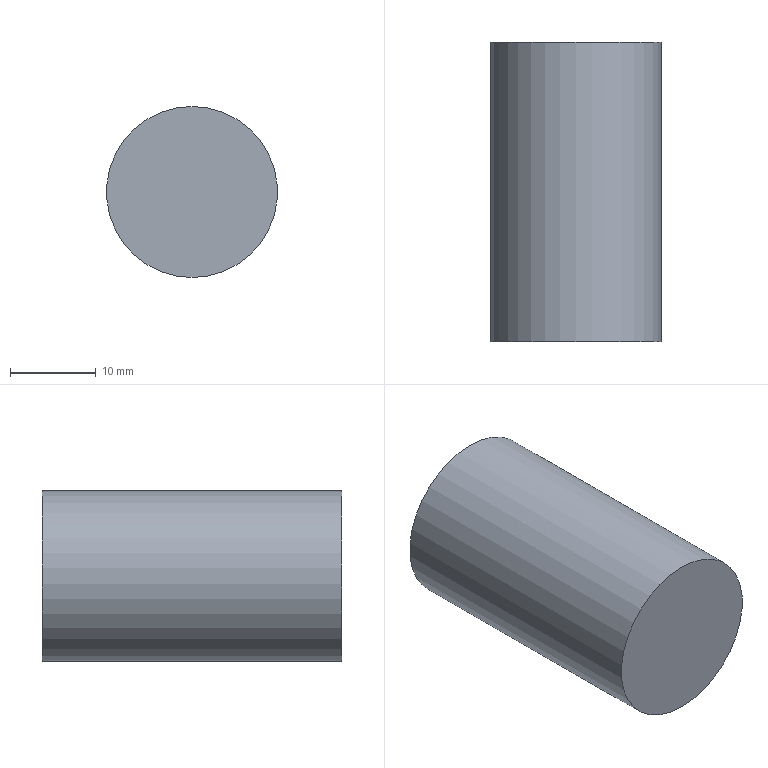Part | STEP file | dijiaolianjie | 1 solid | 3 faces | box 20 x 35 x 20 mm | volume 10996 mm3 | plane 2 | cylinder 1 | commonest cylinder face diameters 20 x1
STEP:
#1=CARTESIAN_POINT('',(0.,0.,0.));
#2=DIRECTION('',(0.,0.,1.));
#3=DIRECTION('',(1.,0.,0.));
#4=AXIS2_PLACEMENT_3D('',#1,#2,#3);
#5=CARTESIAN_POINT('',(0.,35.,10.));
#6=VERTEX_POINT('',#5);
#7=CARTESIAN_POINT('',(0.,35.,0.));
#8=DIRECTION('',(0.,1.,0.));
#9=DIRECTION('',(0.,0.,1.));
#10=AXIS2_PLACEMENT_3D('',#7,#8,#9);
#11=CIRCLE('',#10,10.);
#12=CARTESIAN_POINT('',(0.,35.,0.));
#13=DIRECTION('',(0.,-1.,0.));
#14=DIRECTION('',(0.,0.,-1.));
#15=AXIS2_PLACEMENT_3D('',#12,#13,#14);
#16=CYLINDRICAL_SURFACE('',#15,10.);
#17=CARTESIAN_POINT('',(9.425,0.));
#18=DIRECTION('',(-1.,0.));
#19=VECTOR('',#18,1.);
#20=LINE('',#17,#19);
#21=(GEOMETRIC_REPRESENTATION_CONTEXT(2)PARAMETRIC_REPRESENTATION_CONTEXT()REPRESENTATION_CONTEXT('',''));
#22=DEFINITIONAL_REPRESENTATION('',(#20),#21);
#23=PCURVE('',#16,#22);
#24=CARTESIAN_POINT('',(0.,35.,0.));
#25=DIRECTION('',(0.,1.,0.));
#26=DIRECTION('',(0.,0.,1.));
#27=AXIS2_PLACEMENT_3D('',#24,#25,#26);
#28=PLANE('',#27);
#29=CARTESIAN_POINT('',(0.,0.));
#30=DIRECTION('',(1.,0.));
#31=AXIS2_PLACEMENT_2D('',#29,#30);
#32=CIRCLE('',#31,10.);
#33=(GEOMETRIC_REPRESENTATION_CONTEXT(2)PARAMETRIC_REPRESENTATION_CONTEXT()REPRESENTATION_CONTEXT('',''));
#34=DEFINITIONAL_REPRESENTATION('',(#32),#33);
#35=PCURVE('',#28,#34);
#36=SURFACE_CURVE('',#11,(#23,#35),.PCURVE_S1.);
#37=EDGE_CURVE('',#6,#6,#36,.T.);
#38=ORIENTED_EDGE('',*,*,#37,.F.);
#39=CARTESIAN_POINT('',(0.,0.,10.));
#40=VERTEX_POINT('',#39);
#41=CARTESIAN_POINT('',(0.,35.,10.));
#42=CARTESIAN_POINT('',(0.,0.,10.));
#43=B_SPLINE_CURVE_WITH_KNOTS('',1,(#41,#42),.UNSPECIFIED.,.F.,.F.,(2,2),(0.,35.),.PIECEWISE_BEZIER_KNOTS.);
#44=CARTESIAN_POINT('',(9.425,0.));
#45=DIRECTION('',(0.,1.));
#46=VECTOR('',#45,1.);
#47=LINE('',#44,#46);
#48=(GEOMETRIC_REPRESENTATION_CONTEXT(2)PARAMETRIC_REPRESENTATION_CONTEXT()REPRESENTATION_CONTEXT('',''));
#49=DEFINITIONAL_REPRESENTATION('',(#47),#48);
#50=PCURVE('',#16,#49);
#51=CARTESIAN_POINT('',(3.142,0.));
#52=DIRECTION('',(0.,1.));
#53=VECTOR('',#52,1.);
#54=LINE('',#51,#53);
#55=(GEOMETRIC_REPRESENTATION_CONTEXT(2)PARAMETRIC_REPRESENTATION_CONTEXT()REPRESENTATION_CONTEXT('',''));
#56=DEFINITIONAL_REPRESENTATION('',(#54),#55);
#57=PCURVE('',#16,#56);
#58=SEAM_CURVE('',#43,(#50,#57),.PCURVE_S1.);
#59=EDGE_CURVE('',#6,#40,#58,.T.);
#60=ORIENTED_EDGE('',*,*,#59,.T.);
#61=CARTESIAN_POINT('',(0.,0.,0.));
#62=DIRECTION('',(0.,1.,0.));
#63=DIRECTION('',(0.,0.,1.));
#64=AXIS2_PLACEMENT_3D('',#61,#62,#63);
#65=CIRCLE('',#64,10.);
#66=CARTESIAN_POINT('',(9.425,35.));
#67=DIRECTION('',(-1.,0.));
#68=VECTOR('',#67,1.);
#69=LINE('',#66,#68);
#70=(GEOMETRIC_REPRESENTATION_CONTEXT(2)PARAMETRIC_REPRESENTATION_CONTEXT()REPRESENTATION_CONTEXT('',''));
#71=DEFINITIONAL_REPRESENTATION('',(#69),#70);
#72=PCURVE('',#16,#71);
#73=CARTESIAN_POINT('',(0.,0.,0.));
#74=DIRECTION('',(0.,1.,0.));
#75=DIRECTION('',(0.,0.,1.));
#76=AXIS2_PLACEMENT_3D('',#73,#74,#75);
#77=PLANE('',#76);
#78=CARTESIAN_POINT('',(0.,0.));
#79=DIRECTION('',(1.,0.));
#80=AXIS2_PLACEMENT_2D('',#78,#79);
#81=CIRCLE('',#80,10.);
#82=(GEOMETRIC_REPRESENTATION_CONTEXT(2)PARAMETRIC_REPRESENTATION_CONTEXT()REPRESENTATION_CONTEXT('',''));
#83=DEFINITIONAL_REPRESENTATION('',(#81),#82);
#84=PCURVE('',#77,#83);
#85=SURFACE_CURVE('',#65,(#72,#84),.PCURVE_S1.);
#86=EDGE_CURVE('',#40,#40,#85,.T.);
#87=ORIENTED_EDGE('',*,*,#86,.T.);
#88=ORIENTED_EDGE('',*,*,#59,.F.);
#89=EDGE_LOOP('',(#38,#60,#87,#88));
#90=FACE_BOUND('',#89,.T.);
#91=ADVANCED_FACE('',(#90),#16,.T.);
#92=ORIENTED_EDGE('',*,*,#37,.T.);
#93=EDGE_LOOP('',(#92));
#94=FACE_BOUND('',#93,.T.);
#95=ADVANCED_FACE('',(#94),#28,.T.);
#96=ORIENTED_EDGE('',*,*,#86,.F.);
#97=EDGE_LOOP('',(#96));
#98=FACE_BOUND('',#97,.T.);
#99=ADVANCED_FACE('',(#98),#77,.F.);
#100=CLOSED_SHELL('',(#91,#95,#99));
#101=MANIFOLD_SOLID_BREP('',#100);
#102=(LENGTH_UNIT()NAMED_UNIT(*)SI_UNIT(.MILLI.,.METRE.));
#103=UNCERTAINTY_MEASURE_WITH_UNIT(LENGTH_MEASURE(0.00001),#102,'','');
#104=(NAMED_UNIT(*)PLANE_ANGLE_UNIT()SI_UNIT($,.RADIAN.));
#105=(NAMED_UNIT(*)SI_UNIT($,.STERADIAN.)SOLID_ANGLE_UNIT());
#106=(GEOMETRIC_REPRESENTATION_CONTEXT(3)GLOBAL_UNCERTAINTY_ASSIGNED_CONTEXT((#103))GLOBAL_UNIT_ASSIGNED_CONTEXT((#102,#104,#105))REPRESENTATION_CONTEXT('',''));
#107=ADVANCED_BREP_SHAPE_REPRESENTATION('',(#4,#101),#106);